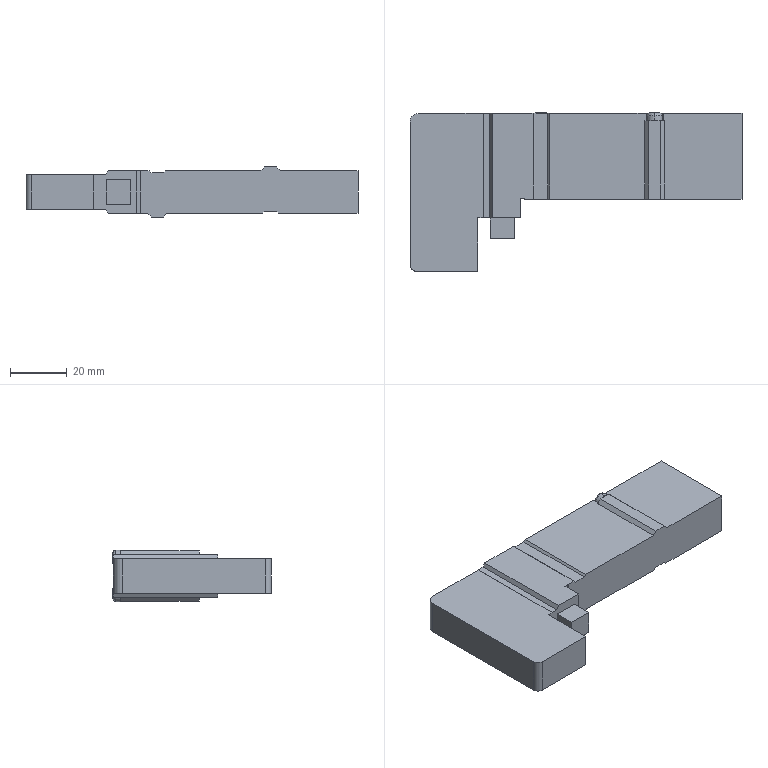Part | SolidWorks | features BaseBody 1 | 1 solid | 225 faces | box 116.6 x 55.58 x 18.1 mm | volume 59586 mm3 | plane 181 | cylinder 40 | spline 4 | commonest cylinder face diameters 1.2 x6 0.8 x4 1 x4 1.5 x4 3.5 x4 5.5 x4